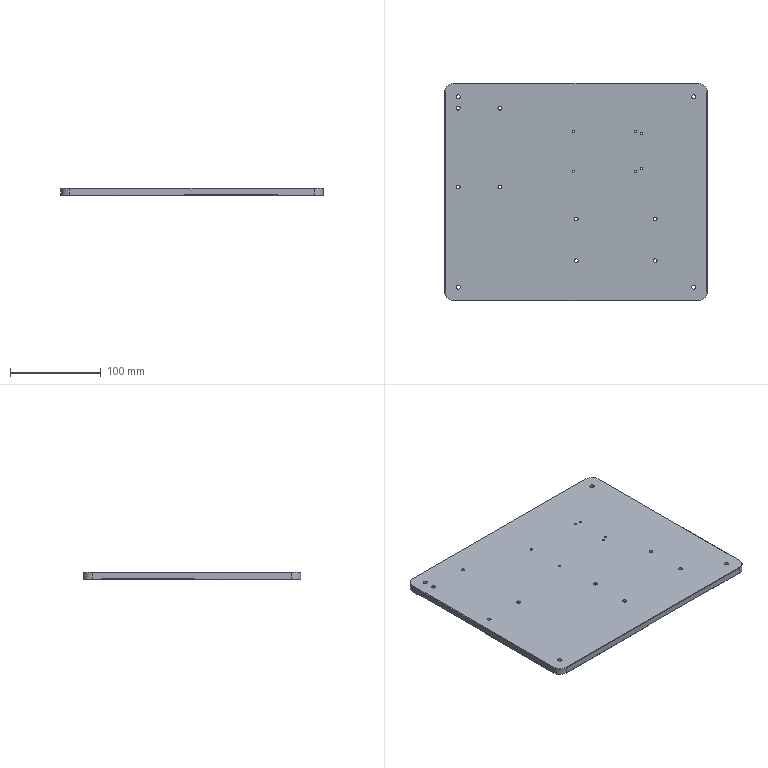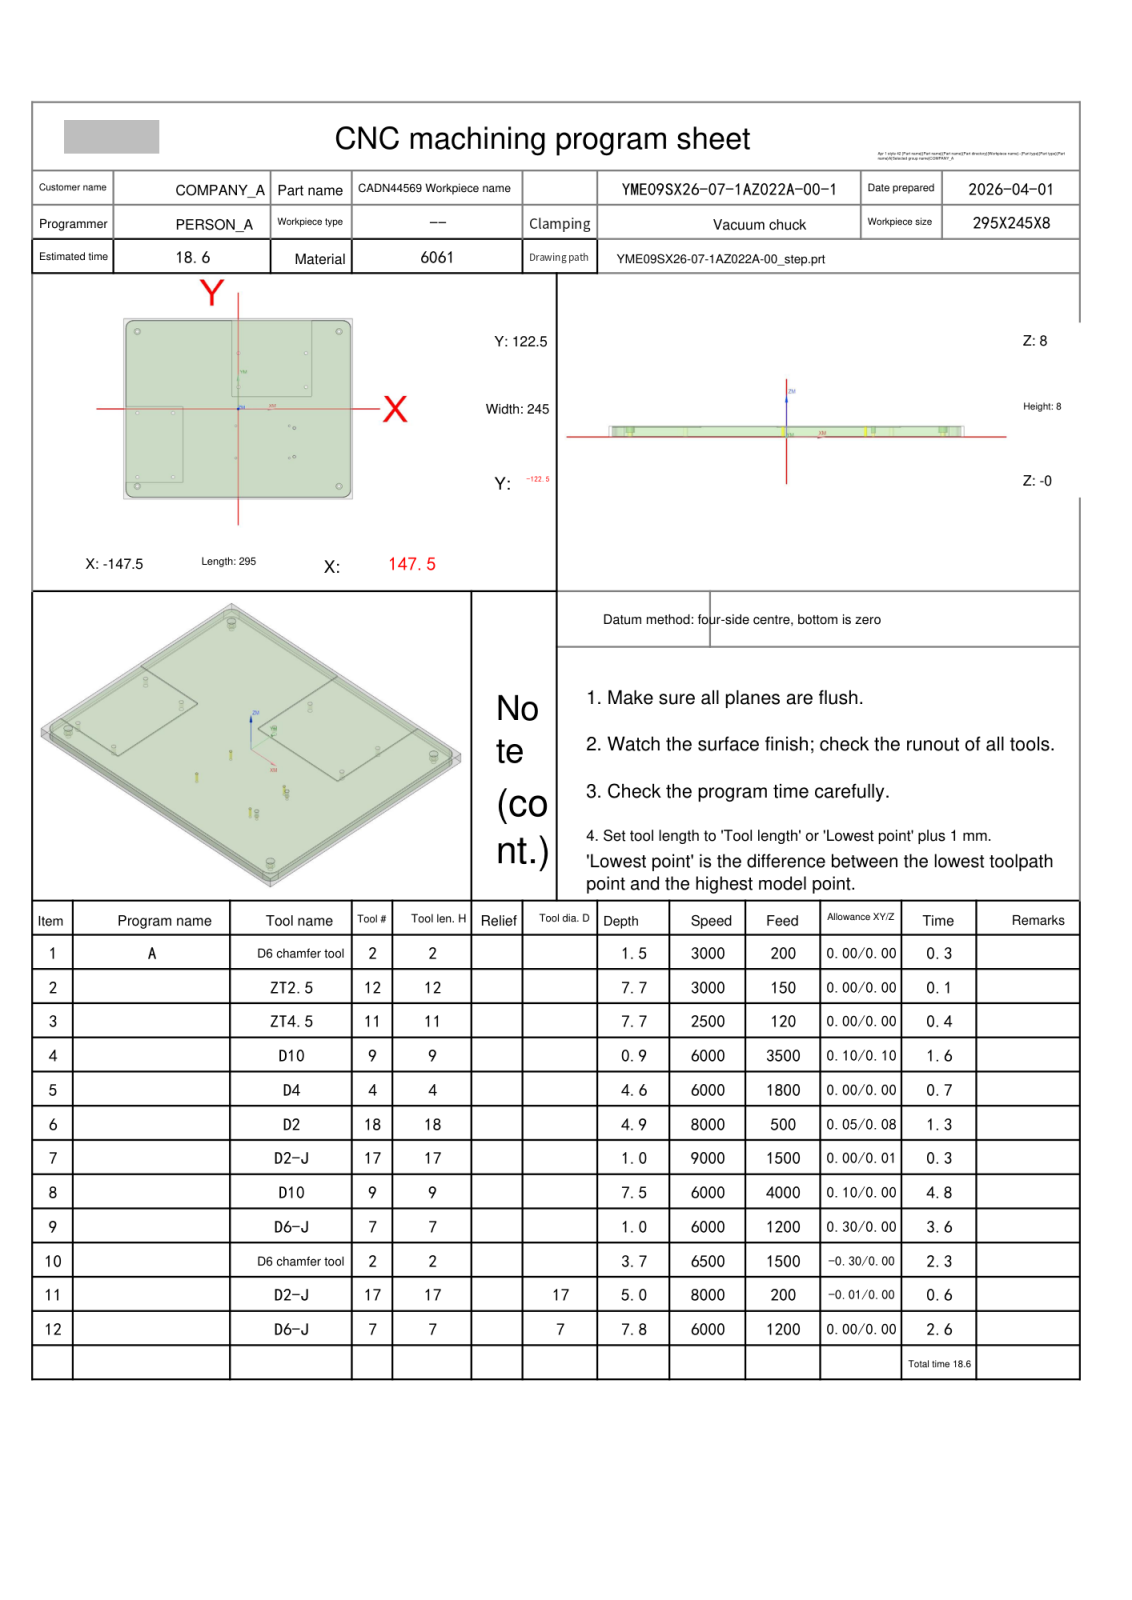NC program | NX | posted by the shop | part box 290 x 240 x 8 mm
Lines 1 to 2078 of 2318, first 1494 of 2076 lines:
%
O0001
(Machine time: 21.04 MIN)
(===Total Tool:8===)
(T2=D6 chamfer tool D=6. R=0. D- H02 Z=4.3   )
(T12=ZT2.5  D=2.5  DR_a=118 D-  H12 Z=0.3   )
(T11=ZT4.5  D=4.5  DR_a=118 D-  H11 Z=0.3   )
(T9=D10     D=10.  R=0.   D-  H09 Z=0.5   )
(T4=D4      D=4.   R=0.   D-  H04 Z=3.4   )
(T18=D2     D=2.   R=0.   D-  H18 Z=3.06  )
(T17=D2-J   D=2.   R=0.   D-  H17 Z=3.    )
(T7=D6-J    D=6.   R=0.   D-  H07 Z=0.2   )
G80 G90 G17 G49 G40
G91 G28 Z0
M01
N1 T02 M06
(D6 chamfer tool D=6. R=0. H=02 ce=0.00 di=0.00)
G00 G90 G54 X-130. Y105. M03 S3000
G43 H02 Z28.
M08
G98 G81 X-130. Y105. Z6.5 R9. F200.
Y-5.5
Y-92.5
Y-105.
X-84. Y-92.5
Y-5.5
X.311 Y29.713
Y75.713
X87.311
X130. Y105.
X87.311 Y29.713
X72.205 Y-25.89
Y-64.89
X130. Y-105.
G80
G00 Z28.
G00 G90 X-3.02 Y-22.984 M03 S3000
Z28.
G98 G81 X-3.02 Y-22.984 Z7. R9. F200.
Y-66.798
X65.704
X65.705 Y-22.984
G80
G00 Z28.
G91 G28 Z0.0
M05
M09
G91 G28 Z0.0
M01
N2 T12 M06
(ZT2.5 D=2.5 DR_a=118 H=12)
G00 G90 G54 X72.205 Y-25.89 M03 S3000
G43 H12 Z28.
M08
G98 G83 X72.205 Y-25.89 Z.3 R9. F150. Q2.
Y-64.89
G80
G00 Z28.
G91 G28 Z0.0
M05
M09
G91 G28 Z0.0
M01
N3 T11 M06
(ZT4.5 D=4.5 DR_a=118 H=11)
G00 G90 G54 X130. Y-105. M03 S2500
G43 H11 Z28.
M08
G98 G83 X130. Y-105. Z.3 R9. F120. Q3.
Y105.
X-130.
Y-105.
G80
G00 Z28.
G91 G28 Z0.0
M05
M09
G91 G28 Z0.0
M01
N4 T09 M06
(D10  D=10. R=0. H=09 ce=0.10 di=0.10)
G00 G90 G54 X38.911 Y71.705 M03 S6000
G43 H09 Z28.
M08
Z8.5
G01 Y63.813 Z8.293 F3500.
X47.711 Z8.063
Y79. Z7.665
X43.311 Z7.55
X38.911
Y63.813
X47.711
Y79.
X43.311
Y86.
X31.911
Y56.813
X54.711
Y86.
X43.311
Y93.
X24.911
Y49.813
X61.711
Y93.
X43.311
Y100.
X17.911
Y42.813
X68.711
Y100.
X43.311
Y107.
X10.911
Y35.813
X75.711
Y107.
X43.311
Y114.
X3.911
Y28.813
X82.711
Y114.
X43.311
Y121.
X-3.089
Y21.813
X89.711
Y121.
X43.311
X42.811
Z8.05
G00 Z8.5
X38.911 Y71.705
Z8.05
G01 Y63.813 Z7.843
X47.711 Z7.613
Y79. Z7.215
X43.311 Z7.1
X38.911
Y63.813
X47.711
Y79.
X43.311
Y86.
X31.911
Y56.813
X54.711
Y86.
X43.311
Y93.
X24.911
Y49.813
X61.711
Y93.
X43.311
Y100.
X17.911
Y42.813
X68.711
Y100.
X43.311
Y107.
X10.911
Y35.813
X75.711
Y107.
X43.311
Y114.
X3.911
Y28.813
X82.711
Y114.
X43.311
Y121.
X-3.089
Y21.813
X89.711
Y121.
X43.311
X42.811
Z7.6
G00 Z28.
G00 G90 X-108.6 Y-52.079 M03 S6000
Z28.
Z8.5
G01 Y-34.6 Z8.042 F3500.
X-113.5 Z7.914
Y-48.5 Z7.55
Y-62.4
X-108.6
Y-34.6
X-113.5
Y-48.5
X-118.
Y-66.9
X-104.1
Y-30.1
X-118.
Y-48.5
X-125.
Y-73.9
X-97.1
Y-23.1
X-125.
Y-48.5
X-132.
Y-80.9
X-90.1
Y-16.1
X-132.
Y-48.5
X-139.
Y-87.9
X-83.1
Y-9.1
X-139.
Y-48.5
X-146.
Y-94.9
X-76.1
Y-2.1
X-146.
Y-48.5
Y-49.
Z8.05
G00 Z8.5
X-108.6 Y-52.079
Z8.05
G01 Y-34.6 Z7.592
X-113.5 Z7.464
Y-48.5 Z7.1
Y-62.4
X-108.6
Y-34.6
X-113.5
Y-48.5
X-118.
Y-66.9
X-104.1
Y-30.1
X-118.
Y-48.5
X-125.
Y-73.9
X-97.1
Y-23.1
X-125.
Y-48.5
X-132.
Y-80.9
X-90.1
Y-16.1
X-132.
Y-48.5
X-139.
Y-87.9
X-83.1
Y-9.1
X-139.
Y-48.5
X-146.
Y-94.9
X-76.1
Y-2.1
X-146.
Y-48.5
Y-49.
Z7.6
G00 Z28.
G91 G28 Z0.0
M05
M09
G91 G28 Z0.0
M01
N5 T04 M06
(D4  D=4. R=0. H=04 ce=0.07 di=0.00)
G00 G90 G54 X-130. Y105. M03 S6000
G43 H04 Z28.
M08
Z8.3
G03 X-129.035 Y104.035 I.965 J0.0 F1800.
X-128.07 Y105. I0.0 J.965
X-128.07 Y105. Z7.95 I-1.93 J0.0
X-128.07 Y105. Z7.6 I-1.93 J0.0
X-128.07 Y105. Z7.25 I-1.93 J0.0
X-128.07 Y105. Z6.9 I-1.93 J0.0
X-128.07 Y105. Z6.55 I-1.93 J0.0
X-128.07 Y105. Z6.2 I-1.93 J0.0
X-128.07 Y105. Z5.85 I-1.93 J0.0
X-128.07 Y105. Z5.5 I-1.93 J0.0
X-128.07 Y105. Z5.15 I-1.93 J0.0
X-128.07 Y105. Z4.8 I-1.93 J0.0
X-128.07 Y105. Z4.45 I-1.93 J0.0
X-128.07 Y105. Z4.1 I-1.93 J0.0
X-128.07 Y105. Z3.75 I-1.93 J0.0
X-128.07 Y105. Z3.4 I-1.93 J0.0
X-130. Y106.93 I-1.93 J0.0
X-131.93 Y105. I0.0 J-1.93
X-130. Y103.07 I1.93 J0.0
X-128.07 Y105. I0.0 J1.93
X-129.035 Y105.965 I-.965 J0.0
X-130. Y105. I0.0 J-.965
G00 Z28.
Y-105.
Z8.3
G03 X-129.035 Y-105.965 I.965 J0.0
X-128.07 Y-105. I0.0 J.965
X-128.07 Y-105. Z7.95 I-1.93 J0.0
X-128.07 Y-105. Z7.6 I-1.93 J0.0
X-128.07 Y-105. Z7.25 I-1.93 J0.0
X-128.07 Y-105. Z6.9 I-1.93 J0.0
X-128.07 Y-105. Z6.55 I-1.93 J0.0
X-128.07 Y-105. Z6.2 I-1.93 J0.0
X-128.07 Y-105. Z5.85 I-1.93 J0.0
X-128.07 Y-105. Z5.5 I-1.93 J0.0
X-128.07 Y-105. Z5.15 I-1.93 J0.0
X-128.07 Y-105. Z4.8 I-1.93 J0.0
X-128.07 Y-105. Z4.45 I-1.93 J0.0
X-128.07 Y-105. Z4.1 I-1.93 J0.0
X-128.07 Y-105. Z3.75 I-1.93 J0.0
X-128.07 Y-105. Z3.4 I-1.93 J0.0
X-130. Y-103.07 I-1.93 J0.0
X-131.93 Y-105. I0.0 J-1.93
X-130. Y-106.93 I1.93 J0.0
X-128.07 Y-105. I0.0 J1.93
X-129.035 Y-104.035 I-.965 J0.0
X-130. Y-105. I0.0 J-.965
G00 Z28.
X130.
Z8.3
G03 X130.965 Y-105.965 I.965 J0.0
X131.93 Y-105. I0.0 J.965
X131.93 Y-105. Z7.95 I-1.93 J0.0
X131.93 Y-105. Z7.6 I-1.93 J0.0
X131.93 Y-105. Z7.25 I-1.93 J0.0
X131.93 Y-105. Z6.9 I-1.93 J0.0
X131.93 Y-105. Z6.55 I-1.93 J0.0
X131.93 Y-105. Z6.2 I-1.93 J0.0
X131.93 Y-105. Z5.85 I-1.93 J0.0
X131.93 Y-105. Z5.5 I-1.93 J0.0
X131.93 Y-105. Z5.15 I-1.93 J0.0
X131.93 Y-105. Z4.8 I-1.93 J0.0
X131.93 Y-105. Z4.45 I-1.93 J0.0
X131.93 Y-105. Z4.1 I-1.93 J0.0
X131.93 Y-105. Z3.75 I-1.93 J0.0
X131.93 Y-105. Z3.4 I-1.93 J0.0
X130. Y-103.07 I-1.93 J0.0
X128.07 Y-105. I0.0 J-1.93
X130. Y-106.93 I1.93 J0.0
X131.93 Y-105. I0.0 J1.93
X130.965 Y-104.035 I-.965 J0.0
X130. Y-105. I0.0 J-.965
G00 Z28.
Y105.
Z8.3
G03 X130.965 Y104.035 I.965 J0.0
X131.93 Y105. I0.0 J.965
X131.93 Y105. Z7.95 I-1.93 J0.0
X131.93 Y105. Z7.6 I-1.93 J0.0
X131.93 Y105. Z7.25 I-1.93 J0.0
X131.93 Y105. Z6.9 I-1.93 J0.0
X131.93 Y105. Z6.55 I-1.93 J0.0
X131.93 Y105. Z6.2 I-1.93 J0.0
X131.93 Y105. Z5.85 I-1.93 J0.0
X131.93 Y105. Z5.5 I-1.93 J0.0
X131.93 Y105. Z5.15 I-1.93 J0.0
X131.93 Y105. Z4.8 I-1.93 J0.0
X131.93 Y105. Z4.45 I-1.93 J0.0
X131.93 Y105. Z4.1 I-1.93 J0.0
X131.93 Y105. Z3.75 I-1.93 J0.0
X131.93 Y105. Z3.4 I-1.93 J0.0
X130. Y106.93 I-1.93 J0.0
X128.07 Y105. I0.0 J-1.93
X130. Y103.07 I1.93 J0.0
X131.93 Y105. I0.0 J1.93
X130.965 Y105.965 I-.965 J0.0
X130. Y105. I0.0 J-.965
G00 Z28.
G00 G90 X-130. Y105. M03 S6000
Z28.
Z3.4
G01 X-128.404 Y104.671 F600.
X-128.336 Y104.664
G03 X-128. Y105. I0.0 J.336
X-130. Y107. I-2. J0.0
X-132. Y105. I0.0 J-2.
X-130. Y103. I2. J0.0
X-128. Y105. I0.0 J2.
X-128.062 Y105.495 I-2. J0.0
X-128.388 Y105.748 I-.325 J-.083
G01 X-128.535 Y105.714
X-130. Y105.
G00 Z28.
Y-105.
Z3.4
G01 X-128.404 Y-105.329
X-128.336 Y-105.336
G03 X-128. Y-105. I0.0 J.336
X-130. Y-103. I-2. J0.0
X-132. Y-105. I0.0 J-2.
X-130. Y-107. I2. J0.0
X-128. Y-105. I0.0 J2.
X-128.062 Y-104.505 I-2. J0.0
X-128.388 Y-104.252 I-.325 J-.083
G01 X-128.535 Y-104.286
X-130. Y-105.
G00 Z28.
X130.
Z3.4
G01 X131.596 Y-105.329
X131.664 Y-105.336
G03 X132. Y-105. I0.0 J.336
X130. Y-103. I-2. J0.0
X128. Y-105. I0.0 J-2.
X130. Y-107. I2. J0.0
X132. Y-105. I0.0 J2.
X131.938 Y-104.505 I-2. J0.0
X131.612 Y-104.252 I-.325 J-.083
G01 X131.465 Y-104.286
X130. Y-105.
G00 Z28.
Y105.
Z3.4
G01 X131.596 Y104.671
X131.664 Y104.664
G03 X132. Y105. I0.0 J.336
X130. Y107. I-2. J0.0
X128. Y105. I0.0 J-2.
X130. Y103. I2. J0.0
X132. Y105. I0.0 J2.
X131.938 Y105.495 I-2. J0.0
X131.612 Y105.748 I-.325 J-.083
G01 X131.465 Y105.714
X130. Y105.
G00 Z28.
G91 G28 Z0.0
M05
M09
G91 G28 Z0.0
M01
N6 T18 M06
(D2  D=2. R=0. H=18 ce=0.05 di=0.08)
G00 G90 G54 X71.255 Y-25.854 M03 S8000
G43 H18 Z28.
M08
Z8.8
G01 Y-26.131 Z8.785 F500.
X71.512 Y-26.583 Z8.758
X71.964 Y-26.84 Z8.731
X72.445 Z8.706
X72.898 Y-26.583 Z8.678
X73.155 Y-26.131 Z8.651
Y-25.65 Z8.626
X73.085 Y-25.46 Z8.615
X72.774 Y-25.093 Z8.59
X72.445 Y-24.94 Z8.571
X71.964 Z8.546
X71.512 Y-25.197 Z8.519
X71.255 Y-25.65 Z8.491
Y-26.131 Z8.466
X71.512 Y-26.583 Z8.439
X71.964 Y-26.84 Z8.412
X72.445 Z8.386
X72.898 Y-26.583 Z8.359
X73.155 Y-26.131 Z8.332
Y-25.65 Z8.307
X73.085 Y-25.46 Z8.296
X72.774 Y-25.093 Z8.271
X72.445 Y-24.94 Z8.252
X71.964 Z8.227
X71.512 Y-25.197 Z8.199
X71.255 Y-25.65 Z8.172
Y-26.131 Z8.147
X71.512 Y-26.583 Z8.12
X71.964 Y-26.84 Z8.092
X72.445 Z8.067
X72.898 Y-26.583 Z8.04
X73.155 Y-26.131 Z8.013
Y-25.89 Z8.
G03 X72.93 Y-25.276 Z7.989 I-.95 J0.0
X72.205 Y-24.94 Z7.975 I-.725 J-.614
X71.255 Y-25.89 Z7.951 I0.0 J-.95
X72.205 Y-26.84 Z7.926 I.95 J0.0
X73.155 Y-25.89 Z7.901 I0.0 J.95
X72.93 Y-25.276 Z7.89 I-.95 J0.0
X72.205 Y-24.94 Z7.877 I-.725 J-.614
X71.255 Y-25.89 Z7.852 I0.0 J-.95
X72.205 Y-26.84 Z7.827 I.95 J0.0
X73.155 Y-25.89 Z7.802 I0.0 J.95
X72.93 Y-25.276 Z7.791 I-.95 J0.0
X72.205 Y-24.94 Z7.778 I-.725 J-.614
X71.255 Y-25.89 Z7.753 I0.0 J-.95
X72.205 Y-26.84 Z7.728 I.95 J0.0
X73.155 Y-25.89 Z7.704 I0.0 J.95
X72.93 Y-25.276 Z7.693 I-.95 J0.0
X72.205 Y-24.94 Z7.679 I-.725 J-.614
X71.255 Y-25.89 Z7.654 I0.0 J-.95
X72.205 Y-26.84 Z7.63 I.95 J0.0
X73.155 Y-25.89 Z7.605 I0.0 J.95
X72.93 Y-25.276 Z7.594 I-.95 J0.0
X72.205 Y-24.94 Z7.58 I-.725 J-.614
X71.255 Y-25.89 Z7.555 I0.0 J-.95
X72.205 Y-26.84 Z7.531 I.95 J0.0
X73.155 Y-25.89 Z7.506 I0.0 J.95
X72.93 Y-25.276 Z7.495 I-.95 J0.0
X72.205 Y-24.94 Z7.481 I-.725 J-.614
X71.255 Y-25.89 Z7.457 I0.0 J-.95
X72.205 Y-26.84 Z7.432 I.95 J0.0
X73.155 Y-25.89 Z7.407 I0.0 J.95
X72.93 Y-25.276 Z7.396 I-.95 J0.0
X72.205 Y-24.94 Z7.383 I-.725 J-.614
X71.255 Y-25.89 Z7.358 I0.0 J-.95
X72.205 Y-26.84 Z7.333 I.95 J0.0
X73.155 Y-25.89 Z7.308 I0.0 J.95
X72.93 Y-25.276 Z7.297 I-.95 J0.0
X72.205 Y-24.94 Z7.284 I-.725 J-.614
X71.255 Y-25.89 Z7.259 I0.0 J-.95
X72.205 Y-26.84 Z7.234 I.95 J0.0
X73.155 Y-25.89 Z7.21 I0.0 J.95
X72.93 Y-25.276 Z7.199 I-.95 J0.0
X72.205 Y-24.94 Z7.185 I-.725 J-.614
X71.255 Y-25.89 Z7.16 I0.0 J-.95
X72.205 Y-26.84 Z7.136 I.95 J0.0
X73.155 Y-25.89 Z7.111 I0.0 J.95
X72.93 Y-25.276 Z7.1 I-.95 J0.0
X72.205 Y-24.94 Z7.086 I-.725 J-.614
X71.255 Y-25.89 Z7.061 I0.0 J-.95
X72.205 Y-26.84 Z7.037 I.95 J0.0
X73.155 Y-25.89 Z7.012 I0.0 J.95
X72.93 Y-25.276 Z7.001 I-.95 J0.0
X72.205 Y-24.94 Z6.987 I-.725 J-.614
X71.255 Y-25.89 Z6.963 I0.0 J-.95
X72.205 Y-26.84 Z6.938 I.95 J0.0
X73.155 Y-25.89 Z6.913 I0.0 J.95
X72.93 Y-25.276 Z6.902 I-.95 J0.0
X72.205 Y-24.94 Z6.889 I-.725 J-.614
X71.255 Y-25.89 Z6.864 I0.0 J-.95
X72.205 Y-26.84 Z6.839 I.95 J0.0
X73.155 Y-25.89 Z6.814 I0.0 J.95
X72.93 Y-25.276 Z6.803 I-.95 J0.0
X72.205 Y-24.94 Z6.79 I-.725 J-.614
X71.255 Y-25.89 Z6.765 I0.0 J-.95
X72.205 Y-26.84 Z6.74 I.95 J0.0
X73.155 Y-25.89 Z6.716 I0.0 J.95
X72.93 Y-25.276 Z6.705 I-.95 J0.0
X72.205 Y-24.94 Z6.691 I-.725 J-.614
X71.255 Y-25.89 Z6.666 I0.0 J-.95
X72.205 Y-26.84 Z6.642 I.95 J0.0
X73.155 Y-25.89 Z6.617 I0.0 J.95
X72.93 Y-25.276 Z6.606 I-.95 J0.0
X72.205 Y-24.94 Z6.592 I-.725 J-.614
X71.255 Y-25.89 Z6.567 I0.0 J-.95
X72.205 Y-26.84 Z6.543 I.95 J0.0
X73.155 Y-25.89 Z6.518 I0.0 J.95
X72.93 Y-25.276 Z6.507 I-.95 J0.0
X72.205 Y-24.94 Z6.493 I-.725 J-.614
X71.255 Y-25.89 Z6.469 I0.0 J-.95
X72.205 Y-26.84 Z6.444 I.95 J0.0
X73.155 Y-25.89 Z6.419 I0.0 J.95
X72.93 Y-25.276 Z6.408 I-.95 J0.0
X72.205 Y-24.94 Z6.395 I-.725 J-.614
X71.255 Y-25.89 Z6.37 I0.0 J-.95
X72.205 Y-26.84 Z6.345 I.95 J0.0
X73.155 Y-25.89 Z6.32 I0.0 J.95
X72.93 Y-25.276 Z6.309 I-.95 J0.0
X72.205 Y-24.94 Z6.296 I-.725 J-.614
X71.255 Y-25.89 Z6.271 I0.0 J-.95
X72.205 Y-26.84 Z6.246 I.95 J0.0
X73.155 Y-25.89 Z6.222 I0.0 J.95
X72.93 Y-25.276 Z6.211 I-.95 J0.0
X72.205 Y-24.94 Z6.197 I-.725 J-.614
X71.255 Y-25.89 Z6.172 I0.0 J-.95
X72.205 Y-26.84 Z6.148 I.95 J0.0
X73.155 Y-25.89 Z6.123 I0.0 J.95
X72.93 Y-25.276 Z6.112 I-.95 J0.0
X72.205 Y-24.94 Z6.098 I-.725 J-.614
X71.255 Y-25.89 Z6.073 I0.0 J-.95
X72.205 Y-26.84 Z6.049 I.95 J0.0
X73.155 Y-25.89 Z6.024 I0.0 J.95
X72.93 Y-25.276 Z6.013 I-.95 J0.0
X72.205 Y-24.94 Z5.999 I-.725 J-.614
X71.255 Y-25.89 Z5.975 I0.0 J-.95
X72.205 Y-26.84 Z5.95 I.95 J0.0
X73.155 Y-25.89 Z5.925 I0.0 J.95
X72.93 Y-25.276 Z5.914 I-.95 J0.0
X72.205 Y-24.94 Z5.901 I-.725 J-.614
X71.255 Y-25.89 Z5.876 I0.0 J-.95
X72.205 Y-26.84 Z5.851 I.95 J0.0
X73.155 Y-25.89 Z5.826 I0.0 J.95
X72.93 Y-25.276 Z5.815 I-.95 J0.0
X72.205 Y-24.94 Z5.802 I-.725 J-.614
X71.255 Y-25.89 Z5.777 I0.0 J-.95
X72.205 Y-26.84 Z5.752 I.95 J0.0
X73.155 Y-25.89 Z5.728 I0.0 J.95
X72.93 Y-25.276 Z5.717 I-.95 J0.0
X72.205 Y-24.94 Z5.703 I-.725 J-.614
X71.255 Y-25.89 Z5.678 I0.0 J-.95
X72.205 Y-26.84 Z5.654 I.95 J0.0
X73.155 Y-25.89 Z5.629 I0.0 J.95
X72.93 Y-25.276 Z5.618 I-.95 J0.0
X72.205 Y-24.94 Z5.604 I-.725 J-.614
X71.255 Y-25.89 Z5.579 I0.0 J-.95
X72.205 Y-26.84 Z5.555 I.95 J0.0
X73.155 Y-25.89 Z5.53 I0.0 J.95
X72.93 Y-25.276 Z5.519 I-.95 J0.0
X72.205 Y-24.94 Z5.505 I-.725 J-.614
X71.255 Y-25.89 Z5.481 I0.0 J-.95
X72.205 Y-26.84 Z5.456 I.95 J0.0
X73.155 Y-25.89 Z5.431 I0.0 J.95
X72.93 Y-25.276 Z5.42 I-.95 J0.0
X72.205 Y-24.94 Z5.407 I-.725 J-.614
X71.255 Y-25.89 Z5.382 I0.0 J-.95
X72.205 Y-26.84 Z5.357 I.95 J0.0
X73.155 Y-25.89 Z5.332 I0.0 J.95
X72.93 Y-25.276 Z5.321 I-.95 J0.0
X72.205 Y-24.94 Z5.308 I-.725 J-.614
X71.255 Y-25.89 Z5.283 I0.0 J-.95
X72.205 Y-26.84 Z5.258 I.95 J0.0
X73.155 Y-25.89 Z5.234 I0.0 J.95
X72.93 Y-25.276 Z5.223 I-.95 J0.0
X72.205 Y-24.94 Z5.209 I-.725 J-.614
X71.255 Y-25.89 Z5.184 I0.0 J-.95
X72.205 Y-26.84 Z5.16 I.95 J0.0
X73.155 Y-25.89 Z5.135 I0.0 J.95
X72.93 Y-25.276 Z5.124 I-.95 J0.0
X72.205 Y-24.94 Z5.11 I-.725 J-.614
X71.255 Y-25.89 Z5.085 I0.0 J-.95
X72.205 Y-26.84 Z5.061 I.95 J0.0
X73.155 Y-25.89 Z5.036 I0.0 J.95
X72.93 Y-25.276 Z5.025 I-.95 J0.0
X72.205 Y-24.94 Z5.011 I-.725 J-.614
X71.255 Y-25.89 Z4.987 I0.0 J-.95
X72.205 Y-26.84 Z4.962 I.95 J0.0
X73.155 Y-25.89 Z4.937 I0.0 J.95
X72.93 Y-25.276 Z4.926 I-.95 J0.0
X72.205 Y-24.94 Z4.913 I-.725 J-.614
X71.255 Y-25.89 Z4.888 I0.0 J-.95
X72.205 Y-26.84 Z4.863 I.95 J0.0
X73.155 Y-25.89 Z4.838 I0.0 J.95
X72.93 Y-25.276 Z4.827 I-.95 J0.0
X72.205 Y-24.94 Z4.814 I-.725 J-.614
X71.255 Y-25.89 Z4.789 I0.0 J-.95
X72.205 Y-26.84 Z4.764 I.95 J0.0
X73.155 Y-25.89 Z4.74 I0.0 J.95
X72.93 Y-25.276 Z4.729 I-.95 J0.0
X72.205 Y-24.94 Z4.715 I-.725 J-.614
X71.255 Y-25.89 Z4.69 I0.0 J-.95
X72.205 Y-26.84 Z4.666 I.95 J0.0
X73.155 Y-25.89 Z4.641 I0.0 J.95
X72.93 Y-25.276 Z4.63 I-.95 J0.0
X72.205 Y-24.94 Z4.616 I-.725 J-.614
X71.255 Y-25.89 Z4.591 I0.0 J-.95
X72.205 Y-26.84 Z4.567 I.95 J0.0
X73.155 Y-25.89 Z4.542 I0.0 J.95
X72.93 Y-25.276 Z4.531 I-.95 J0.0
X72.205 Y-24.94 Z4.517 I-.725 J-.614
X71.255 Y-25.89 Z4.493 I0.0 J-.95
X72.205 Y-26.84 Z4.468 I.95 J0.0
X73.155 Y-25.89 Z4.443 I0.0 J.95
X72.93 Y-25.276 Z4.432 I-.95 J0.0
X72.205 Y-24.94 Z4.419 I-.725 J-.614
X71.255 Y-25.89 Z4.394 I0.0 J-.95
X72.205 Y-26.84 Z4.369 I.95 J0.0
X73.155 Y-25.89 Z4.344 I0.0 J.95
X72.93 Y-25.276 Z4.333 I-.95 J0.0
X72.205 Y-24.94 Z4.32 I-.725 J-.614
X71.255 Y-25.89 Z4.295 I0.0 J-.95
X72.205 Y-26.84 Z4.27 I.95 J0.0
X73.155 Y-25.89 Z4.246 I0.0 J.95
X72.93 Y-25.276 Z4.235 I-.95 J0.0
X72.205 Y-24.94 Z4.221 I-.725 J-.614
X71.255 Y-25.89 Z4.196 I0.0 J-.95
X72.205 Y-26.84 Z4.172 I.95 J0.0
X73.155 Y-25.89 Z4.147 I0.0 J.95
X72.93 Y-25.276 Z4.136 I-.95 J0.0
X72.205 Y-24.94 Z4.122 I-.725 J-.614
X71.255 Y-25.89 Z4.097 I0.0 J-.95
X72.205 Y-26.84 Z4.073 I.95 J0.0
X73.155 Y-25.89 Z4.048 I0.0 J.95
X72.93 Y-25.276 Z4.037 I-.95 J0.0
X72.205 Y-24.94 Z4.023 I-.725 J-.614
X71.255 Y-25.89 Z3.999 I0.0 J-.95
X72.205 Y-26.84 Z3.974 I.95 J0.0
X73.155 Y-25.89 Z3.949 I0.0 J.95
X72.93 Y-25.276 Z3.938 I-.95 J0.0
X72.205 Y-24.94 Z3.925 I-.725 J-.614
X71.255 Y-25.89 Z3.9 I0.0 J-.95
X72.205 Y-26.84 Z3.875 I.95 J0.0
X73.155 Y-25.89 Z3.85 I0.0 J.95
X72.93 Y-25.276 Z3.839 I-.95 J0.0
X72.205 Y-24.94 Z3.826 I-.725 J-.614
X71.255 Y-25.89 Z3.801 I0.0 J-.95
X72.205 Y-26.84 Z3.776 I.95 J0.0
X73.155 Y-25.89 Z3.752 I0.0 J.95
X72.93 Y-25.276 Z3.741 I-.95 J0.0
X72.205 Y-24.94 Z3.727 I-.725 J-.614
X71.255 Y-25.89 Z3.702 I0.0 J-.95
X72.205 Y-26.84 Z3.678 I.95 J0.0
X73.155 Y-25.89 Z3.653 I0.0 J.95
X72.93 Y-25.276 Z3.642 I-.95 J0.0
X72.205 Y-24.94 Z3.628 I-.725 J-.614
X71.255 Y-25.89 Z3.603 I0.0 J-.95
X72.205 Y-26.84 Z3.579 I.95 J0.0
X73.155 Y-25.89 Z3.554 I0.0 J.95
X72.93 Y-25.276 Z3.543 I-.95 J0.0
X72.205 Y-24.94 Z3.529 I-.725 J-.614
X71.255 Y-25.89 Z3.505 I0.0 J-.95
X72.205 Y-26.84 Z3.48 I.95 J0.0
X73.155 Y-25.89 Z3.455 I0.0 J.95
X72.93 Y-25.276 Z3.444 I-.95 J0.0
X72.205 Y-24.94 Z3.431 I-.725 J-.614
X71.255 Y-25.89 Z3.406 I0.0 J-.95
X72.205 Y-26.84 Z3.381 I.95 J0.0
X73.155 Y-25.89 Z3.356 I0.0 J.95
X72.93 Y-25.276 Z3.345 I-.95 J0.0
X72.205 Y-24.94 Z3.332 I-.725 J-.614
X71.255 Y-25.89 Z3.307 I0.0 J-.95
X72.205 Y-26.84 Z3.282 I.95 J0.0
X73.155 Y-25.89 Z3.258 I0.0 J.95
X72.93 Y-25.276 Z3.247 I-.95 J0.0
X72.205 Y-24.94 Z3.233 I-.725 J-.614
X71.255 Y-25.89 Z3.208 I0.0 J-.95
X72.205 Y-26.84 Z3.184 I.95 J0.0
X73.155 Y-25.89 Z3.159 I0.0 J.95
X72.93 Y-25.276 Z3.148 I-.95 J0.0
X72.205 Y-24.94 Z3.134 I-.725 J-.614
X71.255 Y-25.89 Z3.109 I0.0 J-.95
X72.205 Y-26.84 Z3.085 I.95 J0.0
X73.155 Y-25.89 Z3.06 I0.0 J.95
X72.205 Y-24.94 I-.95 J0.0
X71.255 Y-25.89 I0.0 J-.95
X72.205 Y-26.84 I.95 J0.0
X73.155 Y-25.89 I0.0 J.95
X73.072 Y-25.502 I-.95 J0.0
G01 Z3.86
G00 Z28.
X72.252 Y-63.94
Z8.8
G01 X71.964 Z8.785
X71.512 Y-64.197 Z8.758
X71.255 Y-64.65 Z8.73
Y-65.131 Z8.705
X71.512 Y-65.583 Z8.678
X71.964 Y-65.84 Z8.651
X72.445 Z8.625
X72.898 Y-65.583 Z8.598
X73.155 Y-65.131 Z8.571
Y-64.65 Z8.546
X72.898 Y-64.197 Z8.518
X72.445 Y-63.94 Z8.491
X71.964 Z8.466
X71.512 Y-64.197 Z8.439
X71.255 Y-64.65 Z8.411
Y-65.131 Z8.386
X71.512 Y-65.583 Z8.359
X71.964 Y-65.84 Z8.332
X72.445 Z8.306
X72.898 Y-65.583 Z8.279
X73.155 Y-65.131 Z8.252
Y-64.65 Z8.227
X72.898 Y-64.197 Z8.199
X72.445 Y-63.94 Z8.172
X71.964 Z8.147
X71.512 Y-64.197 Z8.12
X71.255 Y-64.65 Z8.092
Y-65.131 Z8.067
X71.512 Y-65.583 Z8.04
X71.964 Y-65.84 Z8.013
X72.205 Z8.
G03 X73.155 Y-64.89 Z7.975 I0.0 J.95
X72.205 Y-63.94 Z7.951 I-.95 J0.0
X71.255 Y-64.89 Z7.926 I0.0 J-.95
X72.205 Y-65.84 Z7.901 I.95 J0.0
X73.155 Y-64.89 Z7.877 I0.0 J.95
X72.205 Y-63.94 Z7.852 I-.95 J0.0
X71.255 Y-64.89 Z7.827 I0.0 J-.95
X72.205 Y-65.84 Z7.802 I.95 J0.0
X73.155 Y-64.89 Z7.778 I0.0 J.95
X72.205 Y-63.94 Z7.753 I-.95 J0.0
X71.255 Y-64.89 Z7.728 I0.0 J-.95
X72.205 Y-65.84 Z7.704 I.95 J0.0
X73.155 Y-64.89 Z7.679 I0.0 J.95
X72.205 Y-63.94 Z7.654 I-.95 J0.0
X71.255 Y-64.89 Z7.63 I0.0 J-.95
X72.205 Y-65.84 Z7.605 I.95 J0.0
X73.155 Y-64.89 Z7.58 I0.0 J.95
X72.205 Y-63.94 Z7.555 I-.95 J0.0
X71.255 Y-64.89 Z7.531 I0.0 J-.95
X72.205 Y-65.84 Z7.506 I.95 J0.0
X73.155 Y-64.89 Z7.481 I0.0 J.95
X72.205 Y-63.94 Z7.457 I-.95 J0.0
X71.255 Y-64.89 Z7.432 I0.0 J-.95
X72.205 Y-65.84 Z7.407 I.95 J0.0
X73.155 Y-64.89 Z7.383 I0.0 J.95
X72.205 Y-63.94 Z7.358 I-.95 J0.0
X71.255 Y-64.89 Z7.333 I0.0 J-.95
X72.205 Y-65.84 Z7.308 I.95 J0.0
X73.155 Y-64.89 Z7.284 I0.0 J.95
X72.205 Y-63.94 Z7.259 I-.95 J0.0
X71.255 Y-64.89 Z7.234 I0.0 J-.95
X72.205 Y-65.84 Z7.21 I.95 J0.0
X73.155 Y-64.89 Z7.185 I0.0 J.95
X72.205 Y-63.94 Z7.16 I-.95 J0.0
X71.255 Y-64.89 Z7.136 I0.0 J-.95
X72.205 Y-65.84 Z7.111 I.95 J0.0
X73.155 Y-64.89 Z7.086 I0.0 J.95
X72.205 Y-63.94 Z7.061 I-.95 J0.0
X71.255 Y-64.89 Z7.037 I0.0 J-.95
X72.205 Y-65.84 Z7.012 I.95 J0.0
X73.155 Y-64.89 Z6.987 I0.0 J.95
X72.205 Y-63.94 Z6.963 I-.95 J0.0
X71.255 Y-64.89 Z6.938 I0.0 J-.95
X72.205 Y-65.84 Z6.913 I.95 J0.0
X73.155 Y-64.89 Z6.889 I0.0 J.95
X72.205 Y-63.94 Z6.864 I-.95 J0.0
X71.255 Y-64.89 Z6.839 I0.0 J-.95
X72.205 Y-65.84 Z6.814 I.95 J0.0
X73.155 Y-64.89 Z6.79 I0.0 J.95
X72.205 Y-63.94 Z6.765 I-.95 J0.0
X71.255 Y-64.89 Z6.74 I0.0 J-.95
X72.205 Y-65.84 Z6.716 I.95 J0.0
X73.155 Y-64.89 Z6.691 I0.0 J.95
X72.205 Y-63.94 Z6.666 I-.95 J0.0
X71.255 Y-64.89 Z6.642 I0.0 J-.95
X72.205 Y-65.84 Z6.617 I.95 J0.0
X73.155 Y-64.89 Z6.592 I0.0 J.95
X72.205 Y-63.94 Z6.567 I-.95 J0.0
X71.255 Y-64.89 Z6.543 I0.0 J-.95
X72.205 Y-65.84 Z6.518 I.95 J0.0
X73.155 Y-64.89 Z6.493 I0.0 J.95
X72.205 Y-63.94 Z6.469 I-.95 J0.0
X71.255 Y-64.89 Z6.444 I0.0 J-.95
X72.205 Y-65.84 Z6.419 I.95 J0.0
X73.155 Y-64.89 Z6.395 I0.0 J.95
X72.205 Y-63.94 Z6.37 I-.95 J0.0
X71.255 Y-64.89 Z6.345 I0.0 J-.95
X72.205 Y-65.84 Z6.32 I.95 J0.0
X73.155 Y-64.89 Z6.296 I0.0 J.95
X72.205 Y-63.94 Z6.271 I-.95 J0.0
X71.255 Y-64.89 Z6.246 I0.0 J-.95
X72.205 Y-65.84 Z6.222 I.95 J0.0
X73.155 Y-64.89 Z6.197 I0.0 J.95
X72.205 Y-63.94 Z6.172 I-.95 J0.0
X71.255 Y-64.89 Z6.148 I0.0 J-.95
X72.205 Y-65.84 Z6.123 I.95 J0.0
X73.155 Y-64.89 Z6.098 I0.0 J.95
X72.205 Y-63.94 Z6.073 I-.95 J0.0
X71.255 Y-64.89 Z6.049 I0.0 J-.95
X72.205 Y-65.84 Z6.024 I.95 J0.0
X73.155 Y-64.89 Z5.999 I0.0 J.95
X72.205 Y-63.94 Z5.975 I-.95 J0.0
X71.255 Y-64.89 Z5.95 I0.0 J-.95
X72.205 Y-65.84 Z5.925 I.95 J0.0
X73.155 Y-64.89 Z5.901 I0.0 J.95
X72.205 Y-63.94 Z5.876 I-.95 J0.0
X71.255 Y-64.89 Z5.851 I0.0 J-.95
X72.205 Y-65.84 Z5.826 I.95 J0.0
X73.155 Y-64.89 Z5.802 I0.0 J.95
X72.205 Y-63.94 Z5.777 I-.95 J0.0
X71.255 Y-64.89 Z5.752 I0.0 J-.95
X72.205 Y-65.84 Z5.728 I.95 J0.0
X73.155 Y-64.89 Z5.703 I0.0 J.95
X72.205 Y-63.94 Z5.678 I-.95 J0.0
X71.255 Y-64.89 Z5.654 I0.0 J-.95
X72.205 Y-65.84 Z5.629 I.95 J0.0
X73.155 Y-64.89 Z5.604 I0.0 J.95
X72.205 Y-63.94 Z5.579 I-.95 J0.0
X71.255 Y-64.89 Z5.555 I0.0 J-.95
X72.205 Y-65.84 Z5.53 I.95 J0.0
X73.155 Y-64.89 Z5.505 I0.0 J.95
X72.205 Y-63.94 Z5.481 I-.95 J0.0
X71.255 Y-64.89 Z5.456 I0.0 J-.95
X72.205 Y-65.84 Z5.431 I.95 J0.0
X73.155 Y-64.89 Z5.407 I0.0 J.95
X72.205 Y-63.94 Z5.382 I-.95 J0.0
X71.255 Y-64.89 Z5.357 I0.0 J-.95
X72.205 Y-65.84 Z5.332 I.95 J0.0
X73.155 Y-64.89 Z5.308 I0.0 J.95
X72.205 Y-63.94 Z5.283 I-.95 J0.0
X71.255 Y-64.89 Z5.258 I0.0 J-.95
X72.205 Y-65.84 Z5.234 I.95 J0.0
X73.155 Y-64.89 Z5.209 I0.0 J.95
X72.205 Y-63.94 Z5.184 I-.95 J0.0
X71.255 Y-64.89 Z5.16 I0.0 J-.95
X72.205 Y-65.84 Z5.135 I.95 J0.0
X73.155 Y-64.89 Z5.11 I0.0 J.95
X72.205 Y-63.94 Z5.085 I-.95 J0.0
X71.255 Y-64.89 Z5.061 I0.0 J-.95
X72.205 Y-65.84 Z5.036 I.95 J0.0
X73.155 Y-64.89 Z5.011 I0.0 J.95
X72.205 Y-63.94 Z4.987 I-.95 J0.0
X71.255 Y-64.89 Z4.962 I0.0 J-.95
X72.205 Y-65.84 Z4.937 I.95 J0.0
X73.155 Y-64.89 Z4.913 I0.0 J.95
X72.205 Y-63.94 Z4.888 I-.95 J0.0
X71.255 Y-64.89 Z4.863 I0.0 J-.95
X72.205 Y-65.84 Z4.838 I.95 J0.0
X73.155 Y-64.89 Z4.814 I0.0 J.95
X72.205 Y-63.94 Z4.789 I-.95 J0.0
X71.255 Y-64.89 Z4.764 I0.0 J-.95
X72.205 Y-65.84 Z4.74 I.95 J0.0
X73.155 Y-64.89 Z4.715 I0.0 J.95
X72.205 Y-63.94 Z4.69 I-.95 J0.0
X71.255 Y-64.89 Z4.666 I0.0 J-.95
X72.205 Y-65.84 Z4.641 I.95 J0.0
X73.155 Y-64.89 Z4.616 I0.0 J.95
X72.205 Y-63.94 Z4.591 I-.95 J0.0
X71.255 Y-64.89 Z4.567 I0.0 J-.95
X72.205 Y-65.84 Z4.542 I.95 J0.0
X73.155 Y-64.89 Z4.517 I0.0 J.95
X72.205 Y-63.94 Z4.493 I-.95 J0.0
X71.255 Y-64.89 Z4.468 I0.0 J-.95
X72.205 Y-65.84 Z4.443 I.95 J0.0
X73.155 Y-64.89 Z4.419 I0.0 J.95
X72.205 Y-63.94 Z4.394 I-.95 J0.0
X71.255 Y-64.89 Z4.369 I0.0 J-.95
X72.205 Y-65.84 Z4.344 I.95 J0.0
X73.155 Y-64.89 Z4.32 I0.0 J.95
X72.205 Y-63.94 Z4.295 I-.95 J0.0
X71.255 Y-64.89 Z4.27 I0.0 J-.95
X72.205 Y-65.84 Z4.246 I.95 J0.0
X73.155 Y-64.89 Z4.221 I0.0 J.95
X72.205 Y-63.94 Z4.196 I-.95 J0.0
X71.255 Y-64.89 Z4.172 I0.0 J-.95
X72.205 Y-65.84 Z4.147 I.95 J0.0
X73.155 Y-64.89 Z4.122 I0.0 J.95
X72.205 Y-63.94 Z4.097 I-.95 J0.0
X71.255 Y-64.89 Z4.073 I0.0 J-.95
X72.205 Y-65.84 Z4.048 I.95 J0.0
X73.155 Y-64.89 Z4.023 I0.0 J.95
X72.205 Y-63.94 Z3.999 I-.95 J0.0
X71.255 Y-64.89 Z3.974 I0.0 J-.95
X72.205 Y-65.84 Z3.949 I.95 J0.0
X73.155 Y-64.89 Z3.925 I0.0 J.95
X72.205 Y-63.94 Z3.9 I-.95 J0.0
X71.255 Y-64.89 Z3.875 I0.0 J-.95
X72.205 Y-65.84 Z3.85 I.95 J0.0
X73.155 Y-64.89 Z3.826 I0.0 J.95
X72.205 Y-63.94 Z3.801 I-.95 J0.0
X71.255 Y-64.89 Z3.776 I0.0 J-.95
X72.205 Y-65.84 Z3.752 I.95 J0.0
X73.155 Y-64.89 Z3.727 I0.0 J.95
X72.205 Y-63.94 Z3.702 I-.95 J0.0
X71.255 Y-64.89 Z3.678 I0.0 J-.95
X72.205 Y-65.84 Z3.653 I.95 J0.0
X73.155 Y-64.89 Z3.628 I0.0 J.95
X72.205 Y-63.94 Z3.603 I-.95 J0.0
X71.255 Y-64.89 Z3.579 I0.0 J-.95
X72.205 Y-65.84 Z3.554 I.95 J0.0
X73.155 Y-64.89 Z3.529 I0.0 J.95
X72.205 Y-63.94 Z3.505 I-.95 J0.0
X71.255 Y-64.89 Z3.48 I0.0 J-.95
X72.205 Y-65.84 Z3.455 I.95 J0.0
X73.155 Y-64.89 Z3.431 I0.0 J.95
X72.205 Y-63.94 Z3.406 I-.95 J0.0
X71.255 Y-64.89 Z3.381 I0.0 J-.95
X72.205 Y-65.84 Z3.356 I.95 J0.0
X73.155 Y-64.89 Z3.332 I0.0 J.95
X72.205 Y-63.94 Z3.307 I-.95 J0.0
X71.255 Y-64.89 Z3.282 I0.0 J-.95
X72.205 Y-65.84 Z3.258 I.95 J0.0
X73.155 Y-64.89 Z3.233 I0.0 J.95
X72.205 Y-63.94 Z3.208 I-.95 J0.0
X71.255 Y-64.89 Z3.184 I0.0 J-.95
X72.205 Y-65.84 Z3.159 I.95 J0.0
X73.155 Y-64.89 Z3.134 I0.0 J.95
X72.205 Y-63.94 Z3.109 I-.95 J0.0
X71.255 Y-64.89 Z3.085 I0.0 J-.95
X72.205 Y-65.84 Z3.06 I.95 J0.0
X73.155 Y-64.89 I0.0 J.95
X72.205 Y-63.94 I-.95 J0.0
X71.255 Y-64.89 I0.0 J-.95
X72.205 Y-65.84 I.95 J0.0
X72.593 Y-65.757 I0.0 J.95
G01 Z3.86
G00 Z28.
G91 G28 Z0.0
M05
M09
G91 G28 Z0.0
M01
N7 T17 M06
(D2-J  D=2. R=0. H=17 ce=0.00 di=0.01)
G00 G90 G54 X-6.444 Y22.69 M03 S9000
G43 H17 Z28.
M08
Z8.608
G01 X-6.454 Y22.686 Z8.494 F1200.
X-6.481 Y22.675 Z8.391
X-6.522 Y22.656 Z8.299
X-6.575 Y22.63 Z8.218
X-6.637 Y22.595 Z8.147
X-6.706 Y22.554 Z8.085
X-6.779 Y22.504 Z8.031
X-6.854 Y22.446 Z7.986
X-6.927 Y22.38 Z7.949
X-6.996 Y22.307 Z7.919
X-7.058 Y22.225 Z7.896
X-7.111 Y22.134 Z7.878
X-7.153 Y22.035 Z7.867
X-7.179 Y21.928 Z7.86
X-7.189 Y21.813 Z7.858
Y17.713 F1500.
X-3.089
X-3.075 Y17.729 Z7.857
X-3.087 Y17.775 Z7.856
X-3.122 Y17.848 Z7.854
X-3.178 Y17.945 Z7.852
X-3.397 Y18.268 Z7.842
X-3.688 Y18.656 Z7.831
X-3.942 Y18.971 Z7.822
X-4.536 Y19.656 Z7.8
X-5.102 Y20.242 Z7.78
X-5.493 Y20.611 Z7.767
X-5.941 Y20.998 Z7.753
X-6.372 Y21.334 Z7.739
X-6.773 Y21.618 Z7.728
X-6.964 Y21.737 Z7.722
X-7.058 Y21.788 Z7.719
X-7.129 Y21.819 Z7.717
X-7.173 Y21.827 Z7.716
X-7.189 Y21.813
Y17.713
X-3.089
X-3.075 Y17.729 Z7.715
X-3.087 Y17.776 Z7.714
X-3.122 Y17.849 Z7.712
X-3.179 Y17.947 Z7.709
X-3.449 Y18.343 Z7.698
X-3.704 Y18.681 Z7.689
X-3.948 Y18.985 Z7.68
X-4.546 Y19.678 Z7.658
X-5.114 Y20.27 Z7.638
X-5.506 Y20.64 Z7.625
X-5.953 Y21.025 Z7.61
X-6.296 Y21.292 Z7.6
X-6.508 Y21.446 Z7.593
X-6.853 Y21.677 Z7.583
X-6.967 Y21.744 Z7.58
X-7.06 Y21.792 Z7.577
X-7.13 Y21.821 Z7.575
X-7.174 Y21.828 Z7.574
X-7.189 Y21.813
Y17.713
X-3.089
X-3.076 Y17.729 Z7.573
X-3.088 Y17.776 Z7.572
X-3.123 Y17.851 Z7.57
X-3.181 Y17.95 Z7.567
X-3.454 Y18.349 Z7.556
X-3.712 Y18.691 Z7.546
X-3.958 Y18.999 Z7.537
X-4.562 Y19.699 Z7.516
X-5.135 Y20.296 Z7.496
X-5.528 Y20.668 Z7.483
X-5.92 Y21.008 Z7.47
X-6.3 Y21.304 Z7.458
X-6.586 Y21.509 Z7.449
X-6.86 Y21.687 Z7.441
X-6.971 Y21.75 Z7.438
X-7.063 Y21.796 Z7.435
X-7.131 Y21.822 Z7.433
X-7.174 Y21.828 Z7.432
X-7.189 Y21.813 Z7.431
Y17.713
X-3.089
X-3.076 Y17.727
X-3.084 Y17.767 Z7.43
X-3.114 Y17.831 Z7.428
X-3.162 Y17.916 Z7.426
X-3.354 Y18.205 Z7.418
X-3.589 Y18.527 Z7.409
X-3.754 Y18.741 Z7.403
X-3.97 Y19.008 Z7.395
X-4.481 Y19.601 Z7.377
X-5.163 Y20.318 Z7.354
X-5.557 Y20.691 Z7.341
X-5.947 Y21.029 Z7.328
X-6.321 Y21.32 Z7.316
X-6.602 Y21.522 Z7.307
X-6.87 Y21.694 Z7.299
X-6.978 Y21.755 Z7.296
X-7.067 Y21.799 Z7.293
X-7.133 Y21.824 Z7.291
X-7.174 Y21.829 Z7.29
X-7.189 Y21.813 Z7.289
Y17.713
X-3.089
X-3.076 Y17.727
X-3.085 Y17.767 Z7.288
X-3.115 Y17.831 Z7.286
X-3.164 Y17.917 Z7.284
X-3.403 Y18.267 Z7.274
X-3.609 Y18.544 Z7.267
X-3.768 Y18.746 Z7.261
X-3.987 Y19.015 Z7.253
X-4.506 Y19.612 Z7.235
X-5.196 Y20.333 Z7.212
X-5.592 Y20.706 Z7.198
X-5.98 Y21.043 Z7.186
X-6.317 Y21.309 Z7.175
X-6.52 Y21.458 Z7.168
X-6.823 Y21.663 Z7.159
X-6.947 Y21.737 Z7.155
X-7.048 Y21.79 Z7.152
X-7.124 Y21.822 Z7.149
X-7.172 Y21.83 Z7.148
X-7.189 Y21.813 Z7.147
Y17.713
X-3.089
X-3.076 Y17.727
X-3.084 Y17.767 Z7.146
X-3.112 Y17.831 Z7.144
X-3.159 Y17.917 Z7.142
X-3.309 Y18.15 Z7.135
X-3.572 Y18.513 Z7.125
X-3.735 Y18.724 Z7.119
X-3.902 Y18.931 Z7.113
X-4.095 Y19.161 Z7.107
X-4.319 Y19.416 Z7.099
X-4.573 Y19.692 Z7.09
X-4.85 Y19.979 Z7.081
X-5.137 Y20.265 Z7.071
X-5.425 Y20.538 Z7.062
X-5.706 Y20.793 Z7.053
X-6.118 Y21.142 Z7.039
X-6.532 Y21.46 Z7.026
X-6.831 Y21.665 Z7.016
X-6.953 Y21.738 Z7.013
X-7.052 Y21.791 Z7.009
X-7.126 Y21.822 Z7.007
X-7.173 Y21.83 Z7.006
X-7.189 Y21.813 Z7.005
Y17.713
X-3.089
X-2.975 Y17.723 Z7.007
X-2.872 Y17.75 Z7.014
X-2.781 Y17.791 Z7.025
X-2.699 Y17.845 Z7.043
X-2.627 Y17.908 Z7.066
X-2.565 Y17.977 Z7.096
X-2.511 Y18.051 Z7.133
X-2.466 Y18.126 Z7.179
X-2.428 Y18.199 Z7.232
X-2.398 Y18.269 Z7.294
X-2.374 Y18.332 Z7.365
X-2.357 Y18.385 Z7.447
X-2.345 Y18.427 Z7.538
X-2.338 Y18.454 Z7.641
X-2.336 Y18.463 Z7.755
G00 Z11.
X88.962
Z8.608
G01 X88.964 Y18.454 Z8.494 F1200.
X88.97 Y18.427 Z8.391
X88.982 Y18.385 Z8.299
X88.999 Y18.332 Z8.218
X89.023 Y18.269 Z8.147
X89.053 Y18.199 Z8.085
X89.09 Y18.126 Z8.031
X89.135 Y18.051 Z7.986
X89.189 Y17.977 Z7.949
X89.251 Y17.908 Z7.919
X89.322 Y17.845 Z7.896
X89.403 Y17.791 Z7.878
X89.495 Y17.75 Z7.867
X89.598 Y17.723 Z7.86
X89.712 Y17.713 Z7.858
X93.811 F1500.
Y21.813
X93.796 Y21.827 Z7.857
X93.751 Y21.815 Z7.856
X93.679 Y21.781 Z7.854
X93.584 Y21.725 Z7.852
X93.267 Y21.506 Z7.842
X92.972 Y21.283 Z7.834
X92.599 Y20.984 Z7.822
X92.01 Y20.467 Z7.803
X91.524 Y20. Z7.787
X91.057 Y19.515 Z7.77
X90.54 Y18.925 Z7.751
X90.241 Y18.552 Z7.74
X90.018 Y18.257 Z7.731
X89.8 Y17.94 Z7.722
X89.744 Y17.845 Z7.719
X89.709 Y17.774 Z7.717
X89.698 Y17.729 Z7.716
X89.712 Y17.713
X93.811
Y21.813
X93.796 Y21.827 Z7.715
X93.751 Y21.815 Z7.714
X93.679 Y21.781 Z7.712
X93.584 Y21.725 Z7.709
X93.267 Y21.506 Z7.7
X92.972 Y21.283 Z7.692
X92.599 Y20.984 Z7.68
X92.01 Y20.467 Z7.661
X91.524 Y20. Z7.645
X91.057 Y19.515 Z7.628
X90.54 Y18.925 Z7.609
X90.241 Y18.552 Z7.598
X90.018 Y18.257 Z7.589
X89.8 Y17.94 Z7.58
X89.744 Y17.845 Z7.577
X89.709 Y17.774 Z7.575
X89.698 Y17.729 Z7.574
X89.712 Y17.713
X93.811
Y21.813
X93.796 Y21.827 Z7.573
X93.751 Y21.815 Z7.572
X93.679 Y21.781 Z7.57
X93.584 Y21.725 Z7.567
X93.267 Y21.506 Z7.558
X92.972 Y21.283 Z7.549
X92.599 Y20.984 Z7.538
X92.01 Y20.467 Z7.519
X91.524 Y20. Z7.503
X91.057 Y19.515 Z7.486
X90.54 Y18.925 Z7.467
X90.241 Y18.552 Z7.456
X90.018 Y18.257 Z7.447
X89.8 Y17.94 Z7.438
X89.744 Y17.845 Z7.435
X89.709 Y17.774 Z7.433
X89.698 Y17.729 Z7.432
X89.712 Y17.713 Z7.431
X93.811
Y21.813
X93.796 Y21.827
X93.751 Y21.815 Z7.43
X93.679 Y21.781 Z7.428
X93.584 Y21.725 Z7.425
X93.267 Y21.506 Z7.416
X92.972 Y21.283 Z7.407
X92.599 Y20.984 Z7.396
X92.01 Y20.467 Z7.377
X91.524 Y20. Z7.36
X91.057 Y19.515 Z7.344
X90.54 Y18.925 Z7.325
X90.241 Y18.552 Z7.313
X90.018 Y18.257 Z7.305
X89.8 Y17.94 Z7.296
X89.744 Y17.845 Z7.293
X89.709 Y17.774 Z7.291
X89.698 Y17.729 Z7.29
X89.712 Y17.713 Z7.289
X93.811
Y21.813
X93.796 Y21.827
X93.751 Y21.815 Z7.288
X93.679 Y21.781 Z7.286
X93.584 Y21.725 Z7.283
X93.267 Y21.507 Z7.274
X92.972 Y21.284 Z7.265
X92.6 Y20.985 Z7.254
X92.01 Y20.468 Z7.235
X91.524 Y20.002 Z7.218
X91.058 Y19.516 Z7.202
X90.54 Y18.926 Z7.183
X90.241 Y18.554 Z7.171
X90.018 Y18.258 Z7.163
X89.8 Y17.94 Z7.153
X89.744 Y17.845 Z7.151
X89.709 Y17.774 Z7.149
X89.698 Y17.729 Z7.148
X89.712 Y17.713 Z7.147
X93.811
Y21.813
X93.796 Y21.827
X93.751 Y21.815 Z7.145
X93.679 Y21.781 Z7.143
X93.584 Y21.725 Z7.141
X93.267 Y21.506 Z7.132
X92.972 Y21.283 Z7.123
X92.599 Y20.984 Z7.112
X92.01 Y20.467 Z7.093
X91.524 Y20. Z7.076
X91.057 Y19.515 Z7.06
X90.54 Y18.925 Z7.041
X90.241 Y18.552 Z7.029
X90.018 Y18.257 Z7.02
X89.8 Y17.94 Z7.011
X89.744 Y17.845 Z7.009
X89.709 Y17.774 Z7.007
X89.698 Y17.729 Z7.005
X89.712 Y17.713
X93.811
Y21.813
X93.802 Y21.927 Z7.007
X93.775 Y22.029 Z7.014
X93.733 Y22.121 Z7.025
X93.68 Y22.202 Z7.043
X93.617 Y22.274 Z7.066
X93.547 Y22.336 Z7.096
X93.474 Y22.389 Z7.133
X93.399 Y22.434 Z7.179
X93.325 Y22.471 Z7.232
X93.256 Y22.501 Z7.294
X93.193 Y22.525 Z7.365
X93.139 Y22.542 Z7.447
X93.098 Y22.554 Z7.538
X93.071 Y22.561 Z7.641
X93.061 Y22.563 Z7.755
G00 Z28.
X-76.849 Y-98.25
Z8.608
G01 X-76.847 Y-98.26 Z8.494 F1200.
X-76.841 Y-98.286 Z8.391
X-76.829 Y-98.328 Z8.299
X-76.812 Y-98.382 Z8.218
X-76.788 Y-98.444 Z8.147
X-76.758 Y-98.514 Z8.085
X-76.721 Y-98.588 Z8.031
X-76.676 Y-98.662 Z7.986
X-76.623 Y-98.736 Z7.949
X-76.561 Y-98.806 Z7.919
X-76.489 Y-98.868 Z7.896
X-76.408 Y-98.922 Z7.878
X-76.316 Y-98.964 Z7.867
X-76.214 Y-98.99 Z7.86
X-76.099 Y-99. Z7.858
X-72. F1500.
Y-94.901
X-72.016 Y-94.887 Z7.857
X-72.061 Y-94.898 Z7.856
X-72.132 Y-94.932 Z7.854
X-72.227 Y-94.988 Z7.852
X-72.544 Y-95.207 Z7.842
X-72.839 Y-95.43 Z7.834
X-73.212 Y-95.729 Z7.822
X-73.802 Y-96.246 Z7.803
X-74.287 Y-96.713 Z7.787
X-74.754 Y-97.198 Z7.77
X-75.271 Y-97.788 Z7.751
X-75.57 Y-98.161 Z7.74
X-75.793 Y-98.456 Z7.731
X-76.012 Y-98.773 Z7.722
X-76.068 Y-98.868 Z7.719
X-76.102 Y-98.939 Z7.717
X-76.113 Y-98.984 Z7.716
X-76.099 Y-99.
X-72.
Y-94.901
X-72.016 Y-94.887 Z7.715
X-72.061 Y-94.898 Z7.714
X-72.132 Y-94.932 Z7.712
X-72.227 Y-94.988 Z7.709
X-72.544 Y-95.207 Z7.7
X-72.839 Y-95.43 Z7.692
X-73.212 Y-95.729 Z7.68
X-73.802 Y-96.246 Z7.661
X-74.287 Y-96.713 Z7.645
X-74.754 Y-97.198 Z7.628
X-75.271 Y-97.788 Z7.609
X-75.57 Y-98.161 Z7.598
X-75.793 Y-98.456 Z7.589
X-76.012 Y-98.773 Z7.58
X-76.068 Y-98.868 Z7.577
X-76.102 Y-98.939 Z7.575
X-76.113 Y-98.984 Z7.574
X-76.099 Y-99.
X-72.
Y-94.901
X-72.016 Y-94.887 Z7.573
X-72.061 Y-94.898 Z7.572
X-72.132 Y-94.932 Z7.57
X-72.227 Y-94.988 Z7.567
X-72.544 Y-95.207 Z7.558
X-72.839 Y-95.43 Z7.549
X-73.212 Y-95.729 Z7.538
X-73.802 Y-96.246 Z7.519
X-74.287 Y-96.713 Z7.503
X-74.754 Y-97.198 Z7.486
X-75.271 Y-97.788 Z7.467
X-75.57 Y-98.161 Z7.456
X-75.793 Y-98.456 Z7.447
X-76.012 Y-98.773 Z7.438
X-76.068 Y-98.868 Z7.435
X-76.102 Y-98.939 Z7.433
X-76.113 Y-98.984 Z7.432
X-76.099 Y-99. Z7.431
X-72.
Y-94.901
X-72.016 Y-94.887
X-72.061 Y-94.898 Z7.43
X-72.132 Y-94.932 Z7.428
X-72.227 Y-94.988 Z7.425
X-72.544 Y-95.207 Z7.416
X-72.839 Y-95.43 Z7.407
X-73.212 Y-95.729 Z7.396
X-73.802 Y-96.246 Z7.377
X-74.287 Y-96.713 Z7.36
X-74.754 Y-97.198 Z7.344
X-75.271 Y-97.788 Z7.325
X-75.57 Y-98.161 Z7.313
X-75.793 Y-98.456 Z7.305
X-76.012 Y-98.773 Z7.296
X-76.068 Y-98.868 Z7.293
X-76.102 Y-98.939 Z7.291
X-76.113 Y-98.984 Z7.29
X-76.099 Y-99. Z7.289
X-72.
Y-94.901
X-72.016 Y-94.887
X-72.061 Y-94.898 Z7.288
X-72.132 Y-94.932 Z7.286
X-72.227 Y-94.988 Z7.283
X-72.544 Y-95.207 Z7.274
X-72.839 Y-95.43 Z7.265
X-73.212 Y-95.729 Z7.254
X-73.802 Y-96.246 Z7.235
X-74.287 Y-96.713 Z7.218
X-74.754 Y-97.198 Z7.202
X-75.271 Y-97.788 Z7.183
X-75.57 Y-98.161 Z7.171
X-75.793 Y-98.456 Z7.163
X-76.012 Y-98.773 Z7.153
X-76.068 Y-98.868 Z7.151
X-76.102 Y-98.939 Z7.149
X-76.113 Y-98.984 Z7.148
X-76.099 Y-99. Z7.147
X-72.
Y-94.901
X-72.016 Y-94.887
X-72.061 Y-94.898 Z7.145
X-72.132 Y-94.932 Z7.143
X-72.227 Y-94.988 Z7.141
X-72.544 Y-95.207 Z7.132
X-72.839 Y-95.43 Z7.123
X-73.212 Y-95.729 Z7.112
X-73.802 Y-96.246 Z7.093
X-74.287 Y-96.713 Z7.076
X-74.754 Y-97.198 Z7.06
X-75.271 Y-97.788 Z7.041
X-75.57 Y-98.161 Z7.029
X-75.793 Y-98.456 Z7.02
X-76.012 Y-98.773 Z7.011
X-76.068 Y-98.868 Z7.009
X-76.102 Y-98.939 Z7.007
X-76.113 Y-98.984 Z7.005
X-76.099 Y-99.
X-72.
Y-94.901
X-72.01 Y-94.786 Z7.007
X-72.036 Y-94.684 Z7.014
X-72.078 Y-94.592 Z7.025
X-72.132 Y-94.511 Z7.043
X-72.194 Y-94.439 Z7.066
X-72.264 Y-94.377 Z7.096
X-72.338 Y-94.324 Z7.133
X-72.412 Y-94.279 Z7.179
X-72.486 Y-94.242 Z7.232
X-72.556 Y-94.212 Z7.294
X-72.618 Y-94.188 Z7.365
X-72.672 Y-94.171 Z7.447
X-72.714 Y-94.159 Z7.538
X-72.74 Y-94.153 Z7.641
X-72.75 Y-94.151 Z7.755
G00 Z11.
Y-2.85
Z8.608
G01 X-72.74 Y-2.847 Z8.494 F1200.
X-72.714 Y-2.841 Z8.391
X-72.672 Y-2.829 Z8.299
X-72.618 Y-2.812 Z8.218
X-72.556 Y-2.788 Z8.147
X-72.486 Y-2.758 Z8.085
X-72.412 Y-2.721 Z8.031
X-72.338 Y-2.676 Z7.986
X-72.264 Y-2.623 Z7.949
X-72.194 Y-2.561 Z7.919
X-72.132 Y-2.489 Z7.896
X-72.078 Y-2.408 Z7.878
X-72.036 Y-2.316 Z7.867
X-72.01 Y-2.214 Z7.86
X-72. Y-2.1 Z7.858
Y2. F1500.
X-76.099
X-76.113 Y1.984 Z7.857
X-76.102 Y1.939 Z7.856
X-76.068 Y1.868 Z7.854
X-76.012 Y1.773 Z7.852
X-75.793 Y1.456 Z7.842
X-75.57 Y1.161 Z7.834
X-75.271 Y.788 Z7.822
X-74.754 Y.198 Z7.803
X-74.287 Y-.287 Z7.787
X-73.802 Y-.754 Z7.77
X-73.212 Y-1.271 Z7.751
X-72.839 Y-1.57 Z7.74
X-72.544 Y-1.793 Z7.731